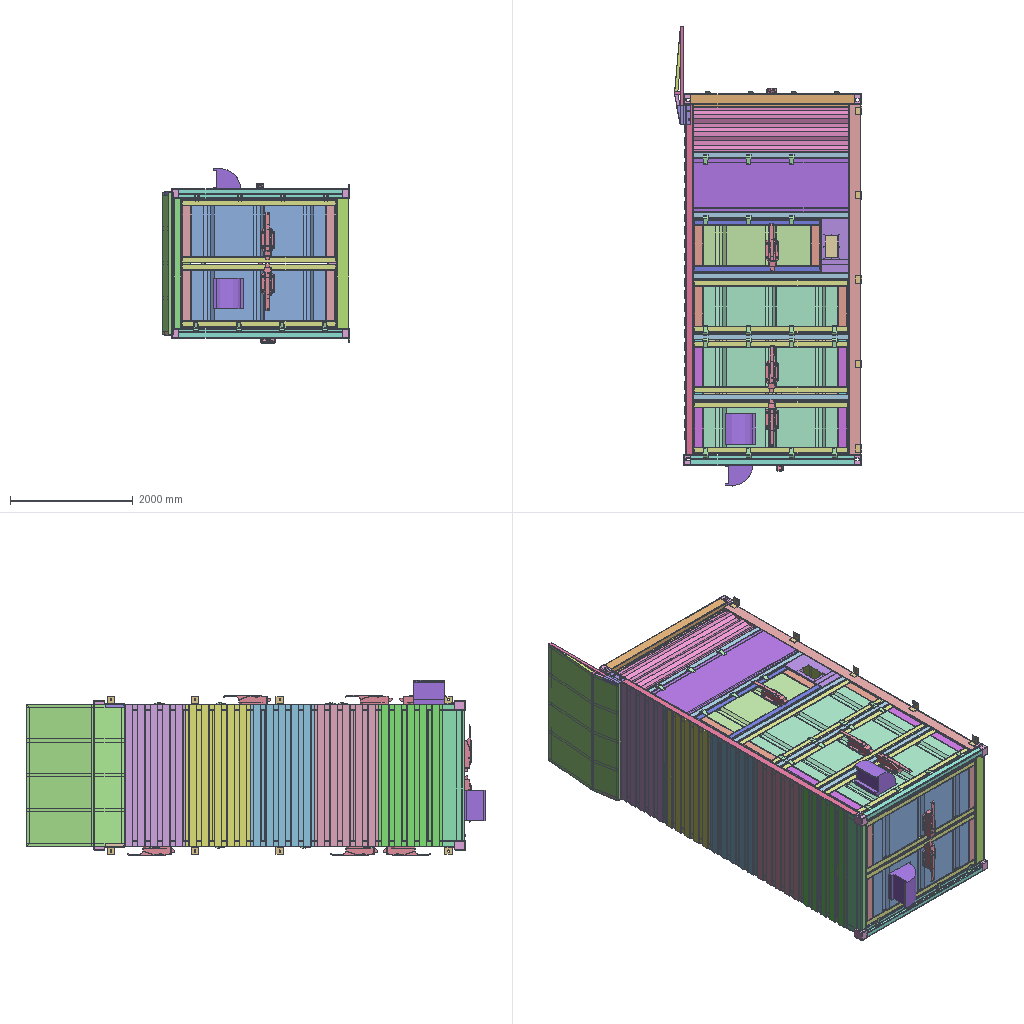Assembly | SolidWorks | 34 different items | 222 placed | box 3046 x 7487 x 2855 mm
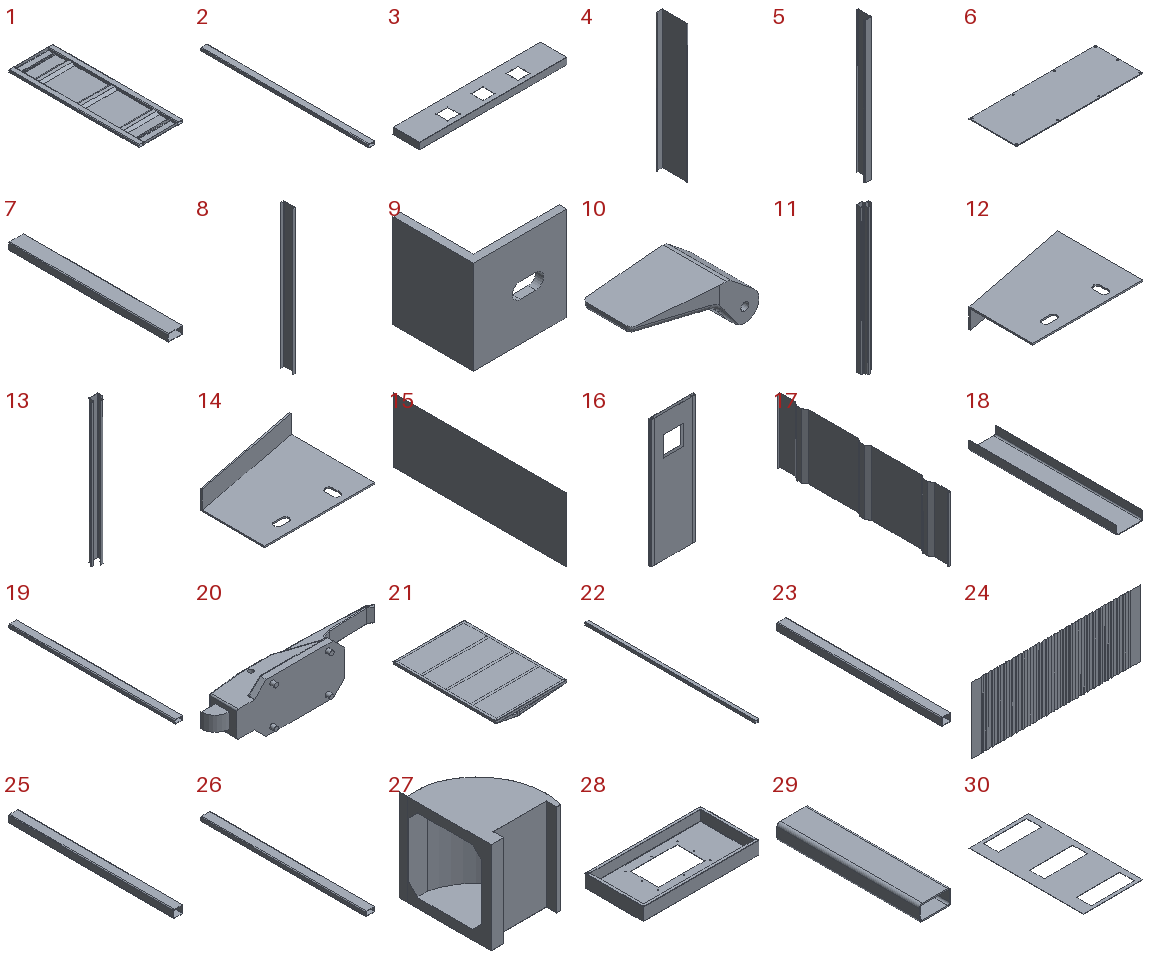Parts list (item | name | quantity | parent item | size | volume | features):
1 | (subassembly) | x11 | - | 845 x 2490 x 50 mm | 7982450 mm3 | -
2 | - | x7 | - | 100 x 2530 x 50 mm | 2735087 mm3 | features ExtruThin 1
3 | - | x1 | - | 2224 x 400.113 x 100 mm | 2783489 mm3 | features EdgeFlange 2, FlatPattern 1, SMBaseFlange 1, SheetMetal 1
4 | - | x1 | - | 100 x 400 x 2130 mm | 2258384 mm3 | features Extrusion 1, FlatPattern 1, SheetMetal 1, SolidToSheetMetal 1
5 | - | x1 | - | 100 x 200 x 2130 mm | 1406384 mm3 | features Extrusion 1, FlatPattern 1, SheetMetal 1, SolidToSheetMetal 1
6 | - | x3 | - | 855.022 x 319.762 x 5 mm | 1363482 mm3 | features Extrusion 1
7 | - | x4 | - | 200 x 2114 x 100 mm | 7153551 mm3 | features ExtruThin 1
8 | - | x18 | - | 50 x 180 x 2124 mm | 2267154 mm3 | features Extrusion 1
9 | - | x10 | - | 120 x 103 x 120 mm | 248458 mm3 | features ExtruThin 1, ICE 1
10 | - | x54 | - | 153 x 80 x 57.284 mm | 267395 mm3 | features Extrusion 1, Fillet 1, ICE 1
11 | - | x2 | - | 174 x 158 x 2660 mm | 7867644 mm3 | features Extrusion 1
12 | - | x1 | - | 300 x 231.743 x 54 mm | 298834 mm3 | features MirrorStock 1
13 | - | x2 | - | 224 x 158 x 2660 mm | 8679415 mm3 | features Extrusion 1
14 | - | x1 | - | 300 x 231.743 x 54 mm | 298834 mm3 | features Extrusion 1, ICE 1
15 | - | x1 | - | 5 x 5744 x 2124 mm | 61001280 mm3 | features Extrusion 1
16 | - | x2 | - | 880 x 51.5 x 2520 mm | 7151820 mm3 | features ICE 2, Extrusion 1
17 | - | x11 | in 1 | 38 x 2190 x 827 mm | 3823055 mm3 | features ExtruThin 1, ICE 1
18 | - | x22 | in 1 | 150 x 827 x 50 mm | 587261 mm3 | features ExtruThin 1
19 | - | x22 | in 1 | 100 x 2040 x 50 mm | 1673251 mm3 | features ExtruThin 1
20 | - | x10 | - | 765.696 x 162.57 x 210 mm | 8155717 mm3 | features BaseBody 5, Scale 1
21 | - | x1 | - | 1604 x 2324 x 150.468 mm | 66441316 mm3 | features WeldCornerFeat 2, 3DProfileFeature 1, BossThin 1, WeldMemberFeat 1, WeldmentFeature 1
22 | - | x2 | - | 120 x 5702 x 100 mm | 9357335 mm3 | features ExtruThin 1
23 | - | x2 | - | 120 x 2114 x 100 mm | 5124111 mm3 | features ExtruThin 1
24 | - | x1 | - | 5925 x 22 x 2324 mm | 31788412 mm3 | features ICE 2, Extrusion 1, LPattern 1
25 | - | x1 | - | 120 x 2124 x 100 mm | 2634230 mm3 | features ExtruThin 1
26 | - | x7 | - | 120 x 2124 x 60 mm | 2805936 mm3 | features ExtruThin 1
27 | - | x2 | - | 386.98 x 495 x 495.029 mm | 841462 mm3 | features Extrusion 1, ICE 1, Shell 1
28 | - | x1 | - | 888 x 450 x 100 mm | 1248625 mm3 | features EdgeFlange 2, FlatPattern 1, SMBaseFlange 1, SheetMetal 1
29 | - | x1 | - | 100 x 446 x 50 mm | 482154 mm3 | features ExtruThin 1
30 | - | x1 | - | 1111 x 2124 x 5 mm | 8464783 mm3 | features Extrusion 1
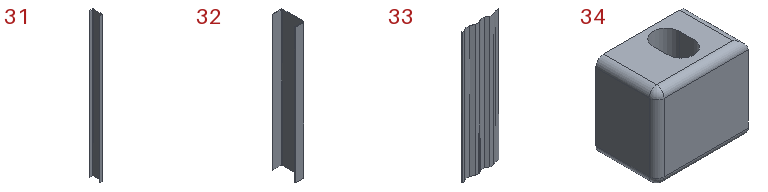31 | - | x3 | - | 50 x 145 x 2124 mm | 1969794 mm3 | features Extrusion 1
32 | - | x6 | - | 60 x 145 x 854 mm | 860318 mm3 | features Extrusion 1
33 | - | x2 | - | 742 x 37.696 x 2530 mm | 4059329 mm3 | features ExtruThin 1
34 | - | x8 | - | 178 x 118 x 162 mm | 2790702 mm3 | features Extrusion 1, Fillet 1
Mates (type | each side: item.copy, entity, surface, feature):
In the top assembly
Coincident | 7.1 plane | assembly plane | 2 times
DistanceDim | 7.1 face plane Extrude-Thin1 | assembly plane
Width | 7.1 face plane Extrude-Thin1 | 7.2 face plane Extrude-Thin1 | 8.1 face plane Boss-Extrude1 | 8.1 face plane Boss-Extrude1
DistanceDim | 8.1 face plane Boss-Extrude1 | 7.2 face plane Extrude-Thin1 | 2 times
Coincident | 8.1 face plane Boss-Extrude1 | 8.2 face plane Boss-Extrude1 | 2 times
DistanceDim | 8.2 face plane Boss-Extrude1 | 8.1 face plane Boss-Extrude1
Coincident | 7.2 face plane Extrude-Thin1 | 7.3 face plane Extrude-Thin1
Width | 7.2 face plane Extrude-Thin1 | 7.1 face plane Extrude-Thin1 | 7.3 face plane Extrude-Thin1 | 7.3 face plane Extrude-Thin1
DistanceDim | 7.3 face plane Extrude-Thin1 | 7.2 face plane Extrude-Thin1
Coincident | 7.2 face plane Extrude-Thin1 | 34.1 face plane Boss-Extrude1
Coincident | 7.3 face plane Extrude-Thin1 | 34.1 face plane Boss-Extrude1
Coincident | 7.4 face plane Extrude-Thin1 | 23.1 face plane Extrude-Thin1
Coincident | 23.1 face plane Extrude-Thin1 | 34.2 face plane Boss-Extrude1
DistanceDim | 23.1 face plane Extrude-Thin1 | 34.2 face plane Boss-Extrude1
Coincident | 34.2 face plane Boss-Extrude1 | 22.1 face plane Extrude-Thin1
Coincident | 23.1 face plane Extrude-Thin1 | 22.1 face plane Extrude-Thin1
Coincident | 7.1 face plane Extrude-Thin1 | 22.1 face plane Extrude-Thin1
Coincident | 26.1 face plane Extrude-Thin1 | 23.1 face plane Extrude-Thin1
Coincident | 26.1 face plane Extrude-Thin1 | 22.1 face plane Extrude-Thin1
DistanceDim | 26.1 face plane Extrude-Thin1 | 34.3 face plane Boss-Extrude1
Coincident | 26.1 face plane Extrude-Thin1 | 26.2 face plane Extrude-Thin1
Coincident | 22.1 face plane Extrude-Thin1 | 26.2 face plane Extrude-Thin1
Coincident | 26.2 face plane Extrude-Thin1 | 26.1 face plane Extrude-Thin1
Coincident | 26.2 face plane Extrude-Thin1 | 26.3 face plane Extrude-Thin1
Coincident | 22.1 face plane Extrude-Thin1 | 26.3 face plane Extrude-Thin1
DistanceDim | 26.3 plane | 34.4 face plane Boss-Extrude1
Coincident | 7.2 face plane Extrude-Thin1 | 2.1 face plane Extrude-Thin1 | 2 times
DistanceDim | 34.1 face plane Boss-Extrude1 | 7.2 face plane Extrude-Thin1
DistanceDim | 2.1 face plane Extrude-Thin1 | 34.1 face plane Boss-Extrude1
Coincident | 7.2 face plane Extrude-Thin1 | 2.2 face plane Extrude-Thin1 | 2 times
DistanceDim | 2.2 face plane Extrude-Thin1 | 2.1 face plane Extrude-Thin1
Coincident | 7.2 face plane Extrude-Thin1 | 2.3 face plane Extrude-Thin1 | 2 times
DistanceDim | 2.3 face plane Extrude-Thin1 | 2.2 face plane Extrude-Thin1
Coincident | 7.2 face plane Extrude-Thin1 | 2.4 face plane Extrude-Thin1 | 2 times
DistanceDim | 2.4 face plane Extrude-Thin1 | 2.3 face plane Extrude-Thin1
Coincident | 7.2 face plane Extrude-Thin1 | 2.5 face plane Extrude-Thin1 | 2 times
DistanceDim | 2.5 face plane Extrude-Thin1 | 2.4 face plane Extrude-Thin1
Coincident | 7.3 face plane Extrude-Thin1 | 11.1 face plane Boss-Extrude1
Coincident | 7.2 face plane Extrude-Thin1 | 11.1 face plane Boss-Extrude1
Coincident | 34.1 face plane Boss-Extrude1 | 11.1 face plane Boss-Extrude1
Coincident | 7.2 face plane Extrude-Thin1 | 13.1 face plane Boss-Extrude1
Coincident | 7.4 face plane Extrude-Thin1 | 13.1 face plane Boss-Extrude1
Coincident | 34.5 face plane Boss-Extrude1 | 13.1 face plane Boss-Extrude1
Width | 11.1 face plane Boss-Extrude1 | 2.1 face plane Extrude-Thin1 | 19.1 face plane Extrude-Thin1 | 19.2 face plane Extrude-Thin1
Width | 7.2 face plane Extrude-Thin1 | 22.2 face plane Extrude-Thin1 | 18.1 face plane Extrude-Thin1 | 18.2 face plane Extrude-Thin1
Coincident | 11.1 face plane Boss-Extrude1 | 19.1 face plane Extrude-Thin1
Width | 7.2 face plane Extrude-Thin1 | 22.2 face plane Extrude-Thin1 | 18.3 face plane Extrude-Thin1 | 18.4 face plane Extrude-Thin1
Coincident | 11.1 face plane Boss-Extrude1 | 19.3 face plane Extrude-Thin1
Width | 2.1 face plane Extrude-Thin1 | 2.2 face plane Extrude-Thin1 | 19.3 face plane Extrude-Thin1 | 19.4 face plane Extrude-Thin1
Width | 7.2 face plane Extrude-Thin1 | 22.2 face plane Extrude-Thin1 | 18.5 face plane Extrude-Thin1 | 18.6 face plane Extrude-Thin1
Coincident | 11.1 face plane Boss-Extrude1 | 19.5 face plane Extrude-Thin1
Width | 2.3 face plane Extrude-Thin1 | 2.2 face plane Extrude-Thin1 | 19.5 face plane Extrude-Thin1 | 19.6 face plane Extrude-Thin1
Coincident | 2.5 face plane Extrude-Thin1 | 33.1 face plane Extrude-Thin1
DistanceDim | 33.1 face plane Extrude-Thin1 | 2.5 face plane Extrude-Thin1
Coincident | 7.2 face plane Extrude-Thin1 | 33.1 face plane Extrude-Thin1
Coincident | 11.1 face plane Boss-Extrude1 | 19.7 face plane Extrude-Thin1
Width | 2.3 face plane Extrude-Thin1 | 2.4 face plane Extrude-Thin1 | 19.7 face plane Extrude-Thin1 | 19.8 face plane Extrude-Thin1
Coincident | 7.1 face plane Extrude-Thin1 | 2.6 face plane Extrude-Thin1 | 2 times
DistanceDim | 2.6 face plane Extrude-Thin1 | 34.6 face plane Boss-Extrude1
Coincident | 7.1 face plane Extrude-Thin1 | 2.7 face plane Extrude-Thin1 | 2 times
DistanceDim | 2.7 face plane Extrude-Thin1 | 2.6 face plane Extrude-Thin1
Coincident | 18.6 face plane Extrude-Thin1 | 18.7 face plane Extrude-Thin1
Coincident | 18.2 face plane Extrude-Thin1 | 18.8 face plane Extrude-Thin1
Coincident | 7.1 face plane Extrude-Thin1 | 19.9 face plane Extrude-Thin1
DistanceDim | 19.10 face plane Extrude-Thin1 | 11.2 face plane Boss-Extrude1
Coincident | 7.1 face plane Extrude-Thin1 | 19.11 face plane Extrude-Thin1
Coincident | 18.2 face plane Extrude-Thin1 | 18.9 face plane Extrude-Thin1
DistanceDim | 19.12 face plane Extrude-Thin1 | 19.9 face plane Extrude-Thin1
Coincident | 18.2 face plane Extrude-Thin1 | 18.10 face plane Extrude-Thin1
Coincident | 7.1 face plane Extrude-Thin1 | 19.13 face plane Extrude-Thin1
DistanceDim | 19.14 face plane Extrude-Thin1 | 19.11 face plane Extrude-Thin1
Width | 2.3 face plane Extrude-Thin1 | 2.4 face plane Extrude-Thin1 | 28.1 face plane Edge-Flange1 | 28.1 face plane Edge-Flange1
Coincident | 7.2 face plane Extrude-Thin1 | 28.1 face plane Base-Flange1
Coincident | 7.2 face plane Extrude-Thin1 | 28.1 face plane Edge-Flange1
Coincident | 28.1 face plane Base-Flange1 | 29.1 face plane Extrude-Thin1
DistanceDim | 29.1 face plane Extrude-Thin1 | 28.1 face plane Edge-Flange1
Coincident | 28.1 face plane Edge-Flange1 | 29.1 face plane Extrude-Thin1
Coincident | 18.11 face plane Extrude-Thin1 | 18.12 face plane Extrude-Thin1
Coincident | 7.3 face plane Extrude-Thin1 | 18.12 face plane Extrude-Thin1
DistanceDim | 19.15 face plane Extrude-Thin1 | 11.2 face plane Boss-Extrude1
Coincident | 15.1 face plane Boss-Extrude1 | 31.1 face plane Boss-Extrude1
Width | 7.1 face plane Extrude-Thin1 | 7.2 face plane Extrude-Thin1 | 31.1 face plane Boss-Extrude1 | 31.1 face plane Boss-Extrude1
Coincident | 15.1 face plane Boss-Extrude1 | 31.2 face plane Boss-Extrude1
Coincident | 31.1 face plane Boss-Extrude1 | 31.2 face plane Boss-Extrude1
DistanceDim | 31.2 face plane Boss-Extrude1 | 7.4 face plane Extrude-Thin1
DistanceDim | 31.2 face plane Boss-Extrude1 | 31.1 face plane Boss-Extrude1
Coincident | 31.1 face plane Boss-Extrude1 | 31.3 face plane Boss-Extrude1 | 2 times
DistanceDim | 31.3 face plane Boss-Extrude1 | 31.1 face plane Boss-Extrude1
Coincident | 31.1 face plane Boss-Extrude1 | 30.1 face plane Boss-Extrude1 | 2 times
Coincident | 31.3 face plane Boss-Extrude1 | 30.1 face plane Boss-Extrude1
Coincident | 30.1 face plane Boss-Extrude1 | 6.1 face plane Boss-Extrude1
Width | 6.1 face plane Boss-Extrude1 | 6.1 face plane Boss-Extrude1 | 30.1 face plane Boss-Extrude1 | 30.1 face plane Boss-Extrude1 | 2 times
Coincident | 30.1 face plane Boss-Extrude1 | 6.2 face plane Boss-Extrude1
Width | 6.2 face plane Boss-Extrude1 | 6.2 face plane Boss-Extrude1 | 30.1 face plane Boss-Extrude1 | 30.1 face plane Boss-Extrude1 | 2 times
Coincident | 30.1 face plane Boss-Extrude1 | 6.3 face plane Boss-Extrude1
Width | 6.3 face plane Boss-Extrude1 | 6.3 face plane Boss-Extrude1 | 30.1 face plane Boss-Extrude1 | 30.1 face plane Boss-Extrude1 | 2 times
Coincident | 22.2 face plane Extrude-Thin1 | 25.1 face plane Extrude-Thin1 | 2 times
Coincident | 2.4 face plane Extrude-Thin1 | 25.1 face plane Extrude-Thin1
Coincident | 34.7 face plane Boss-Extrude1 | 21.1 face plane Extrude-Thin1
Width | 13.1 face plane Boss-Extrude1 | 13.2 face plane Boss-Extrude1 | 21.1 face plane Square bar 50(7) | 21.1 face plane Square bar 50(7)
DistanceDim | 34.2 face plane Boss-Extrude1 | 21.1 face plane Extrude-Thin1
Width | 2.4 face plane Extrude-Thin1 | 2.5 face plane Extrude-Thin1 | 16.1 face plane Boss-Extrude1 | 16.1 face plane Boss-Extrude1
Coincident | 7.2 face plane Extrude-Thin1 | 16.1 face plane Boss-Extrude1
DistanceDim | 22.2 face plane Extrude-Thin1 | 16.1 face plane Boss-Extrude1
Coincident | 21.1 face plane Square bar 50(7) | 14.1 face plane Boss-Extrude1
Coincident | 21.1 face plane Extrude-Thin1 | 14.1 face plane Boss-Extrude2
DistanceDim | 14.1 edge | 34.2 face plane Boss-Extrude1
Coincident | 22.2 face plane Extrude-Thin1 | 24.1 face plane LPattern1
DistanceDim | 24.1 face plane LPattern1 | 23.1 face plane Extrude-Thin1
Width | 22.2 face plane Extrude-Thin1 | 22.1 face plane Extrude-Thin1 | 24.1 face plane Boss-Extrude1 | 24.1 face plane Boss-Extrude1
Coincident | 31.1 face plane Boss-Extrude1 | 32.1 face plane Boss-Extrude1
Coincident | 31.3 face plane Boss-Extrude1 | 32.1 face plane Boss-Extrude1 | 2 times
Coincident | 32.1 face plane Boss-Extrude1 | 32.2 face plane Boss-Extrude1 | 2 times
DistanceDim | 32.2 face plane Boss-Extrude1 | 32.1 face plane Boss-Extrude1
Coincident | 25.1 face plane Extrude-Thin1 | 3.1 face plane Edge-Flange1
Coincident | 25.1 face plane Extrude-Thin1 | 3.1 face plane Base-Flange1
Width | 22.2 face plane Extrude-Thin1 | 22.1 face plane Extrude-Thin1 | 3.1 face plane Edge-Flange1 | 3.1 face plane Edge-Flange1
Coincident | 2.7 face plane Extrude-Thin1 | 5.1 face plane Convert entities 1
Coincident | 3.1 face plane Base-Flange1 | 5.1 face plane Convert entities 1
Coincident | 3.1 face plane Edge-Flange1 | 5.1 face plane Convert entities 1
Coincident | 2.4 face plane Extrude-Thin1 | 4.1 face plane Convert entities 1
Coincident | 3.1 face plane Base-Flange1 | 4.1 face plane Convert entities 1
Coincident | 3.1 face plane Edge-Flange1 | 4.1 face plane Convert entities 1
Coincident | 7.1 face plane Extrude-Thin1 | 9.1 face plane Extrude-Thin1
Coincident | 34.6 face plane Boss-Extrude1 | 9.1 face plane Extrude-Thin1
DistanceDim | 9.1 face plane Extrude-Thin1 | 34.6 face plane Boss-Extrude1
Coincident | 17.1 face plane Extrude-Thin1 | 27.1 face plane Boss-Extrude1
DistanceDim | 27.1 face plane Boss-Extrude1 | 17.1 face plane Extrude-Thin1
Coincident | 19.16 face plane Extrude-Thin1 | 10.1 face plane Boss-Extrude1
Coincident | 19.1 face plane Extrude-Thin1 | 10.2 face plane Boss-Extrude1
DistanceDim | 10.2 face plane Boss-Extrude1 | 19.1 face plane Extrude-Thin1
Coincident | 19.10 face plane Extrude-Thin1 | 10.3 face plane Boss-Extrude1
Coincident | 2.6 face plane Extrude-Thin1 | 10.4 face plane Boss-Extrude1
DistanceDim | 10.4 face plane Boss-Extrude1 | 22.1 face plane Extrude-Thin1
DistanceDim | 23.1 face plane Extrude-Thin1 | 10.1 face plane Boss-Extrude1
Tangent | 10.5 face cylinder Boss-Extrude1 | 19.17 face plane Extrude-Thin1
DistanceDim | 10.5 face plane Boss-Extrude1 | 23.1 face plane Extrude-Thin1
Coincident | 2.1 face plane Extrude-Thin1 | 20.1 face plane Door lock-1-solid1
Parallel | 22.2 face plane Extrude-Thin1 | 20.1 face plane Door lock-1-solid1
Coincident | 19.18 face plane Extrude-Thin1 | 20.2 face plane Door lock-1-solid1
Coincident | 19.19 face plane Extrude-Thin1 | 20.3 face plane Door lock-1-solid1
Parallel | 7.4 face plane Extrude-Thin1 | 20.3 face plane Door lock-1-solid1
Coincident | 20.4 face plane Door lock-1-solid1 | 16.2 face plane Boss-Extrude1
Coincident | 17.2 face plane Extrude-Thin1 | 20.5 face plane Door lock-1-solid1
Coincident | 19.12 face plane Extrude-Thin1 | 20.6 face plane Door lock-1-solid1
In subassembly 1
Coincident | 19.20 face plane Extrude-Thin1 | 18.13 face plane Extrude-Thin1 | 3 times
Coincident | 19.20 face plane Extrude-Thin1 | 18.14 face plane Extrude-Thin1 | 3 times
Coincident | 19.20 face plane Extrude-Thin1 | 17.3 face plane Extrude-Thin1 | 2 times
Coincident | 18.13 face plane Extrude-Thin1 | 19.21 face plane Extrude-Thin1 | 3 times
Coincident | 18.13 face plane Extrude-Thin1 | 17.3 face plane Extrude-Thin1